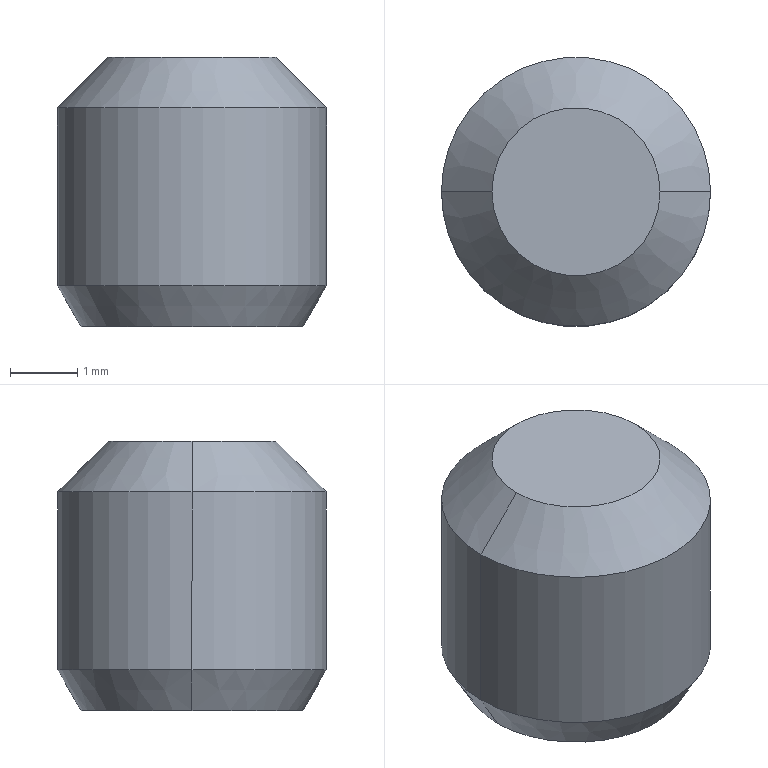Part | SolidWorks | features BaseBody 1 | 1 solid | 15 faces | box 4 x 4 x 4 mm | volume 40.721 mm3 | plane 9 | cone 4 | cylinder 2 | commonest cylinder face diameters 4 x2
STEP:
#1=CARTESIAN_POINT('',(461.064,-93.168,231.151));
#2=VERTEX_POINT('',#1);
#3=CARTESIAN_POINT('',(457.064,-93.168,231.151));
#4=VERTEX_POINT('',#3);
#5=CARTESIAN_POINT('',(459.064,-93.168,231.151));
#6=DIRECTION('',(0.000000024,-0.000000004,1.));
#7=DIRECTION('',(1.,0.,-0.000000024));
#8=AXIS2_PLACEMENT_3D('',#5,#6,#7);
#9=CIRCLE('',#8,2.);
#10=EDGE_CURVE('',#2,#4,#9,.T.);
#11=ORIENTED_EDGE('',*,*,#10,.T.);
#12=CARTESIAN_POINT('',(457.064,-93.168,233.795));
#13=VERTEX_POINT('',#12);
#14=CARTESIAN_POINT('',(457.064,-93.168,232.473));
#15=DIRECTION('',(0.000000024,-0.000000004,1.));
#16=VECTOR('',#15,1000.);
#17=LINE('',#14,#16);
#18=EDGE_CURVE('',#4,#13,#17,.T.);
#19=ORIENTED_EDGE('',*,*,#18,.T.);
#20=CARTESIAN_POINT('',(461.064,-93.168,233.795));
#21=VERTEX_POINT('',#20);
#22=CARTESIAN_POINT('',(459.064,-93.168,233.795));
#23=DIRECTION('',(-0.000000024,0.000000004,-1.));
#24=DIRECTION('',(1.,0.,-0.000000024));
#25=AXIS2_PLACEMENT_3D('',#22,#23,#24);
#26=CIRCLE('',#25,2.);
#27=EDGE_CURVE('',#13,#21,#26,.T.);
#28=ORIENTED_EDGE('',*,*,#27,.T.);
#29=CARTESIAN_POINT('',(461.064,-93.168,232.473));
#30=DIRECTION('',(0.000000024,-0.000000004,1.));
#31=VECTOR('',#30,1000.);
#32=LINE('',#29,#31);
#33=EDGE_CURVE('',#2,#21,#32,.T.);
#34=ORIENTED_EDGE('',*,*,#33,.F.);
#35=EDGE_LOOP('',(#11,#19,#28,#34));
#36=FACE_OUTER_BOUND('',#35,.T.);
#37=CARTESIAN_POINT('',(459.064,-93.168,232.473));
#38=DIRECTION('',(0.000000024,-0.000000004,1.));
#39=DIRECTION('',(1.,0.,-0.000000024));
#40=AXIS2_PLACEMENT_3D('',#37,#38,#39);
#41=CYLINDRICAL_SURFACE('',#40,2.);
#42=ADVANCED_FACE('',(#36),#41,.T.);
#43=CARTESIAN_POINT('',(460.714,-93.168,230.545));
#44=VERTEX_POINT('',#43);
#45=CARTESIAN_POINT('',(457.414,-93.168,230.545));
#46=VERTEX_POINT('',#45);
#47=CARTESIAN_POINT('',(459.064,-93.168,230.545));
#48=DIRECTION('',(0.000000024,-0.000000004,1.));
#49=DIRECTION('',(1.,0.,-0.000000024));
#50=AXIS2_PLACEMENT_3D('',#47,#48,#49);
#51=CIRCLE('',#50,1.65);
#52=EDGE_CURVE('',#44,#46,#51,.T.);
#53=ORIENTED_EDGE('',*,*,#52,.T.);
#54=CARTESIAN_POINT('',(457.064,-93.168,231.151));
#55=DIRECTION('',(-0.5,-0.000000003,0.866));
#56=VECTOR('',#55,1000.);
#57=LINE('',#54,#56);
#58=EDGE_CURVE('',#46,#4,#57,.T.);
#59=ORIENTED_EDGE('',*,*,#58,.T.);
#60=ORIENTED_EDGE('',*,*,#10,.F.);
#61=CARTESIAN_POINT('',(461.064,-93.168,231.151));
#62=DIRECTION('',(0.5,-0.000000003,0.866));
#63=VECTOR('',#62,1000.);
#64=LINE('',#61,#63);
#65=EDGE_CURVE('',#44,#2,#64,.T.);
#66=ORIENTED_EDGE('',*,*,#65,.F.);
#67=EDGE_LOOP('',(#53,#59,#60,#66));
#68=FACE_OUTER_BOUND('',#67,.T.);
#69=CARTESIAN_POINT('',(459.064,-93.168,231.151));
#70=DIRECTION('',(0.000000024,-0.000000004,1.));
#71=DIRECTION('',(1.,0.,-0.000000024));
#72=AXIS2_PLACEMENT_3D('',#69,#70,#71);
#73=CONICAL_SURFACE('',#72,2.,0.5236);
#74=ADVANCED_FACE('',(#68),#73,.T.);
#75=CARTESIAN_POINT('',(457.814,-93.168,234.545));
#76=VERTEX_POINT('',#75);
#77=CARTESIAN_POINT('',(460.314,-93.168,234.545));
#78=VERTEX_POINT('',#77);
#79=CARTESIAN_POINT('',(459.064,-93.168,234.545));
#80=DIRECTION('',(-0.000000024,0.000000004,-1.));
#81=DIRECTION('',(-1.,0.,0.000000024));
#82=AXIS2_PLACEMENT_3D('',#79,#80,#81);
#83=CIRCLE('',#82,1.25);
#84=EDGE_CURVE('',#76,#78,#83,.T.);
#85=ORIENTED_EDGE('',*,*,#84,.T.);
#86=CARTESIAN_POINT('',(461.064,-93.168,233.795));
#87=DIRECTION('',(0.7071,0.000000003,-0.7071));
#88=VECTOR('',#87,1000.);
#89=LINE('',#86,#88);
#90=EDGE_CURVE('',#78,#21,#89,.T.);
#91=ORIENTED_EDGE('',*,*,#90,.T.);
#92=ORIENTED_EDGE('',*,*,#27,.F.);
#93=CARTESIAN_POINT('',(457.064,-93.168,233.795));
#94=DIRECTION('',(-0.7071,0.000000003,-0.7071));
#95=VECTOR('',#94,1000.);
#96=LINE('',#93,#95);
#97=EDGE_CURVE('',#76,#13,#96,.T.);
#98=ORIENTED_EDGE('',*,*,#97,.F.);
#99=EDGE_LOOP('',(#85,#91,#92,#98));
#100=FACE_OUTER_BOUND('',#99,.T.);
#101=CARTESIAN_POINT('',(459.064,-93.168,233.795));
#102=DIRECTION('',(-0.000000024,0.000000004,-1.));
#103=DIRECTION('',(-1.,0.,0.000000024));
#104=AXIS2_PLACEMENT_3D('',#101,#102,#103);
#105=CONICAL_SURFACE('',#104,2.,0.7854);
#106=ADVANCED_FACE('',(#100),#105,.T.);
#107=ORIENTED_EDGE('',*,*,#18,.F.);
#108=CARTESIAN_POINT('',(459.064,-93.168,231.151));
#109=DIRECTION('',(0.000000024,-0.000000004,1.));
#110=DIRECTION('',(1.,0.,-0.000000024));
#111=AXIS2_PLACEMENT_3D('',#108,#109,#110);
#112=CIRCLE('',#111,2.);
#113=EDGE_CURVE('',#4,#2,#112,.T.);
#114=ORIENTED_EDGE('',*,*,#113,.T.);
#115=ORIENTED_EDGE('',*,*,#33,.T.);
#116=CARTESIAN_POINT('',(459.064,-93.168,233.795));
#117=DIRECTION('',(-0.000000024,0.000000004,-1.));
#118=DIRECTION('',(1.,0.,-0.000000024));
#119=AXIS2_PLACEMENT_3D('',#116,#117,#118);
#120=CIRCLE('',#119,2.);
#121=EDGE_CURVE('',#21,#13,#120,.T.);
#122=ORIENTED_EDGE('',*,*,#121,.T.);
#123=EDGE_LOOP('',(#107,#114,#115,#122));
#124=FACE_OUTER_BOUND('',#123,.T.);
#125=CARTESIAN_POINT('',(459.064,-93.168,232.473));
#126=DIRECTION('',(0.000000024,-0.000000004,1.));
#127=DIRECTION('',(1.,0.,-0.000000024));
#128=AXIS2_PLACEMENT_3D('',#125,#126,#127);
#129=CYLINDRICAL_SURFACE('',#128,2.);
#130=ADVANCED_FACE('',(#124),#129,.T.);
#131=ORIENTED_EDGE('',*,*,#58,.F.);
#132=CARTESIAN_POINT('',(459.064,-93.168,230.545));
#133=DIRECTION('',(0.000000024,-0.000000004,1.));
#134=DIRECTION('',(1.,0.,-0.000000024));
#135=AXIS2_PLACEMENT_3D('',#132,#133,#134);
#136=CIRCLE('',#135,1.65);
#137=EDGE_CURVE('',#46,#44,#136,.T.);
#138=ORIENTED_EDGE('',*,*,#137,.T.);
#139=ORIENTED_EDGE('',*,*,#65,.T.);
#140=ORIENTED_EDGE('',*,*,#113,.F.);
#141=EDGE_LOOP('',(#131,#138,#139,#140));
#142=FACE_OUTER_BOUND('',#141,.T.);
#143=CARTESIAN_POINT('',(459.064,-93.168,231.151));
#144=DIRECTION('',(0.000000024,-0.000000004,1.));
#145=DIRECTION('',(1.,0.,-0.000000024));
#146=AXIS2_PLACEMENT_3D('',#143,#144,#145);
#147=CONICAL_SURFACE('',#146,2.,0.5236);
#148=ADVANCED_FACE('',(#142),#147,.T.);
#149=ORIENTED_EDGE('',*,*,#90,.F.);
#150=CARTESIAN_POINT('',(459.064,-93.168,234.545));
#151=DIRECTION('',(-0.000000024,0.000000004,-1.));
#152=DIRECTION('',(-1.,0.,0.000000024));
#153=AXIS2_PLACEMENT_3D('',#150,#151,#152);
#154=CIRCLE('',#153,1.25);
#155=EDGE_CURVE('',#78,#76,#154,.T.);
#156=ORIENTED_EDGE('',*,*,#155,.T.);
#157=ORIENTED_EDGE('',*,*,#97,.T.);
#158=ORIENTED_EDGE('',*,*,#121,.F.);
#159=EDGE_LOOP('',(#149,#156,#157,#158));
#160=FACE_OUTER_BOUND('',#159,.T.);
#161=CARTESIAN_POINT('',(459.064,-93.168,233.795));
#162=DIRECTION('',(-0.000000024,0.000000004,-1.));
#163=DIRECTION('',(-1.,0.,0.000000024));
#164=AXIS2_PLACEMENT_3D('',#161,#162,#163);
#165=CONICAL_SURFACE('',#164,2.,0.7854);
#166=ADVANCED_FACE('',(#160),#165,.T.);
#167=ORIENTED_EDGE('',*,*,#52,.F.);
#168=ORIENTED_EDGE('',*,*,#137,.F.);
#169=EDGE_LOOP('',(#167,#168));
#170=FACE_OUTER_BOUND('',#169,.T.);
#171=CARTESIAN_POINT('',(458.881,-94.308,230.545));
#172=VERTEX_POINT('',#171);
#173=CARTESIAN_POINT('',(459.959,-93.896,230.545));
#174=VERTEX_POINT('',#173);
#175=CARTESIAN_POINT('',(458.881,-94.308,230.545));
#176=DIRECTION('',(0.9343,0.3564,-0.000000021));
#177=VECTOR('',#176,1000.);
#178=LINE('',#175,#177);
#179=EDGE_CURVE('',#172,#174,#178,.T.);
#180=ORIENTED_EDGE('',*,*,#179,.T.);
#181=CARTESIAN_POINT('',(460.142,-92.756,230.545));
#182=VERTEX_POINT('',#181);
#183=CARTESIAN_POINT('',(459.959,-93.896,230.545));
#184=DIRECTION('',(0.1585,0.9874,0.));
#185=VECTOR('',#184,1000.);
#186=LINE('',#183,#185);
#187=EDGE_CURVE('',#174,#182,#186,.T.);
#188=ORIENTED_EDGE('',*,*,#187,.T.);
#189=CARTESIAN_POINT('',(459.247,-92.027,230.545));
#190=VERTEX_POINT('',#189);
#191=CARTESIAN_POINT('',(460.142,-92.756,230.545));
#192=DIRECTION('',(-0.7758,0.6309,0.000000021));
#193=VECTOR('',#192,1000.);
#194=LINE('',#191,#193);
#195=EDGE_CURVE('',#182,#190,#194,.T.);
#196=ORIENTED_EDGE('',*,*,#195,.T.);
#197=CARTESIAN_POINT('',(458.168,-92.439,230.545));
#198=VERTEX_POINT('',#197);
#199=CARTESIAN_POINT('',(459.247,-92.027,230.545));
#200=DIRECTION('',(-0.9343,-0.3564,0.000000021));
#201=VECTOR('',#200,1000.);
#202=LINE('',#199,#201);
#203=EDGE_CURVE('',#190,#198,#202,.T.);
#204=ORIENTED_EDGE('',*,*,#203,.T.);
#205=CARTESIAN_POINT('',(457.985,-93.579,230.545));
#206=VERTEX_POINT('',#205);
#207=CARTESIAN_POINT('',(458.168,-92.439,230.545));
#208=DIRECTION('',(-0.1585,-0.9874,0.));
#209=VECTOR('',#208,1000.);
#210=LINE('',#207,#209);
#211=EDGE_CURVE('',#198,#206,#210,.T.);
#212=ORIENTED_EDGE('',*,*,#211,.T.);
#213=CARTESIAN_POINT('',(457.985,-93.579,230.545));
#214=DIRECTION('',(0.7758,-0.6309,-0.000000021));
#215=VECTOR('',#214,1000.);
#216=LINE('',#213,#215);
#217=EDGE_CURVE('',#206,#172,#216,.T.);
#218=ORIENTED_EDGE('',*,*,#217,.T.);
#219=EDGE_LOOP('',(#180,#188,#196,#204,#212,#218));
#220=FACE_BOUND('',#219,.T.);
#221=CARTESIAN_POINT('',(458.423,-92.647,230.545));
#222=DIRECTION('',(-0.000000024,0.000000004,-1.));
#223=DIRECTION('',(-1.,0.,0.000000024));
#224=AXIS2_PLACEMENT_3D('',#221,#222,#223);
#225=PLANE('',#224);
#226=ADVANCED_FACE('',(#170,#220),#225,.T.);
#227=ORIENTED_EDGE('',*,*,#84,.F.);
#228=ORIENTED_EDGE('',*,*,#155,.F.);
#229=EDGE_LOOP('',(#227,#228));
#230=FACE_OUTER_BOUND('',#229,.T.);
#231=CARTESIAN_POINT('',(458.579,-92.773,234.545));
#232=DIRECTION('',(0.000000024,-0.000000004,1.));
#233=DIRECTION('',(1.,0.,-0.000000024));
#234=AXIS2_PLACEMENT_3D('',#231,#232,#233);
#235=PLANE('',#234);
#236=ADVANCED_FACE('',(#230),#235,.T.);
#237=CARTESIAN_POINT('',(460.142,-92.756,232.045));
#238=VERTEX_POINT('',#237);
#239=CARTESIAN_POINT('',(460.142,-92.756,230.545));
#240=DIRECTION('',(0.000000024,-0.000000004,1.));
#241=VECTOR('',#240,1000.);
#242=LINE('',#239,#241);
#243=EDGE_CURVE('',#182,#238,#242,.T.);
#244=ORIENTED_EDGE('',*,*,#243,.F.);
#245=ORIENTED_EDGE('',*,*,#187,.F.);
#246=CARTESIAN_POINT('',(459.959,-93.896,232.045));
#247=VERTEX_POINT('',#246);
#248=CARTESIAN_POINT('',(459.959,-93.896,230.545));
#249=DIRECTION('',(-0.000000024,0.000000004,-1.));
#250=VECTOR('',#249,1000.);
#251=LINE('',#248,#250);
#252=EDGE_CURVE('',#247,#174,#251,.T.);
#253=ORIENTED_EDGE('',*,*,#252,.F.);
#254=CARTESIAN_POINT('',(460.142,-92.756,232.045));
#255=DIRECTION('',(-0.1585,-0.9874,0.));
#256=VECTOR('',#255,1000.);
#257=LINE('',#254,#256);
#258=EDGE_CURVE('',#238,#247,#257,.T.);
#259=ORIENTED_EDGE('',*,*,#258,.F.);
#260=EDGE_LOOP('',(#244,#245,#253,#259));
#261=FACE_OUTER_BOUND('',#260,.T.);
#262=CARTESIAN_POINT('',(460.142,-92.756,230.545));
#263=DIRECTION('',(0.9874,-0.1585,-0.000000024));
#264=DIRECTION('',(0.1585,0.9874,0.));
#265=AXIS2_PLACEMENT_3D('',#262,#263,#264);
#266=PLANE('',#265);
#267=ADVANCED_FACE('',(#261),#266,.F.);
#268=ORIENTED_EDGE('',*,*,#252,.T.);
#269=ORIENTED_EDGE('',*,*,#179,.F.);
#270=CARTESIAN_POINT('',(458.881,-94.308,232.045));
#271=VERTEX_POINT('',#270);
#272=CARTESIAN_POINT('',(458.881,-94.308,230.545));
#273=DIRECTION('',(-0.000000004,0.000000011,-1.));
#274=VECTOR('',#273,1000.);
#275=LINE('',#272,#274);
#276=EDGE_CURVE('',#271,#172,#275,.T.);
#277=ORIENTED_EDGE('',*,*,#276,.F.);
#278=CARTESIAN_POINT('',(459.959,-93.896,232.045));
#279=DIRECTION('',(-0.9343,-0.3564,0.));
#280=VECTOR('',#279,1000.);
#281=LINE('',#278,#280);
#282=EDGE_CURVE('',#247,#271,#281,.T.);
#283=ORIENTED_EDGE('',*,*,#282,.F.);
#284=EDGE_LOOP('',(#268,#269,#277,#283));
#285=FACE_OUTER_BOUND('',#284,.T.);
#286=CARTESIAN_POINT('',(459.959,-93.896,230.545));
#287=DIRECTION('',(0.3564,-0.9343,-0.000000012));
#288=DIRECTION('',(0.9343,0.3564,0.));
#289=AXIS2_PLACEMENT_3D('',#286,#287,#288);
#290=PLANE('',#289);
#291=ADVANCED_FACE('',(#285),#290,.F.);
#292=ORIENTED_EDGE('',*,*,#276,.T.);
#293=ORIENTED_EDGE('',*,*,#217,.F.);
#294=CARTESIAN_POINT('',(457.985,-93.579,232.045));
#295=VERTEX_POINT('',#294);
#296=CARTESIAN_POINT('',(457.985,-93.579,230.545));
#297=DIRECTION('',(-0.000000008,-0.000000009,-1.));
#298=VECTOR('',#297,1000.);
#299=LINE('',#296,#298);
#300=EDGE_CURVE('',#295,#206,#299,.T.);
#301=ORIENTED_EDGE('',*,*,#300,.F.);
#302=CARTESIAN_POINT('',(458.881,-94.308,232.045));
#303=DIRECTION('',(-0.7758,0.6309,0.));
#304=VECTOR('',#303,1000.);
#305=LINE('',#302,#304);
#306=EDGE_CURVE('',#271,#295,#305,.T.);
#307=ORIENTED_EDGE('',*,*,#306,.F.);
#308=EDGE_LOOP('',(#292,#293,#301,#307));
#309=FACE_OUTER_BOUND('',#308,.T.);
#310=CARTESIAN_POINT('',(458.881,-94.308,230.545));
#311=DIRECTION('',(-0.6309,-0.7758,0.000000012));
#312=DIRECTION('',(0.7758,-0.6309,0.));
#313=AXIS2_PLACEMENT_3D('',#310,#311,#312);
#314=PLANE('',#313);
#315=ADVANCED_FACE('',(#309),#314,.F.);
#316=ORIENTED_EDGE('',*,*,#300,.T.);
#317=ORIENTED_EDGE('',*,*,#211,.F.);
#318=CARTESIAN_POINT('',(458.168,-92.439,232.045));
#319=VERTEX_POINT('',#318);
#320=CARTESIAN_POINT('',(458.168,-92.439,230.545));
#321=DIRECTION('',(-0.000000024,0.000000004,-1.));
#322=VECTOR('',#321,1000.);
#323=LINE('',#320,#322);
#324=EDGE_CURVE('',#319,#198,#323,.T.);
#325=ORIENTED_EDGE('',*,*,#324,.F.);
#326=CARTESIAN_POINT('',(457.985,-93.579,232.045));
#327=DIRECTION('',(0.1585,0.9874,0.));
#328=VECTOR('',#327,1000.);
#329=LINE('',#326,#328);
#330=EDGE_CURVE('',#295,#319,#329,.T.);
#331=ORIENTED_EDGE('',*,*,#330,.F.);
#332=EDGE_LOOP('',(#316,#317,#325,#331));
#333=FACE_OUTER_BOUND('',#332,.T.);
#334=CARTESIAN_POINT('',(457.985,-93.579,230.545));
#335=DIRECTION('',(-0.9874,0.1585,0.000000024));
#336=DIRECTION('',(-0.1585,-0.9874,0.));
#337=AXIS2_PLACEMENT_3D('',#334,#335,#336);
#338=PLANE('',#337);
#339=ADVANCED_FACE('',(#333),#338,.F.);
#340=ORIENTED_EDGE('',*,*,#324,.T.);
#341=ORIENTED_EDGE('',*,*,#203,.F.);
#342=CARTESIAN_POINT('',(459.247,-92.027,232.045));
#343=VERTEX_POINT('',#342);
#344=CARTESIAN_POINT('',(459.247,-92.027,230.545));
#345=DIRECTION('',(-0.000000004,0.000000011,-1.));
#346=VECTOR('',#345,1000.);
#347=LINE('',#344,#346);
#348=EDGE_CURVE('',#343,#190,#347,.T.);
#349=ORIENTED_EDGE('',*,*,#348,.F.);
#350=CARTESIAN_POINT('',(458.168,-92.439,232.045));
#351=DIRECTION('',(0.9343,0.3564,0.));
#352=VECTOR('',#351,1000.);
#353=LINE('',#350,#352);
#354=EDGE_CURVE('',#319,#343,#353,.T.);
#355=ORIENTED_EDGE('',*,*,#354,.F.);
#356=EDGE_LOOP('',(#340,#341,#349,#355));
#357=FACE_OUTER_BOUND('',#356,.T.);
#358=CARTESIAN_POINT('',(458.168,-92.439,230.545));
#359=DIRECTION('',(-0.3564,0.9343,0.000000012));
#360=DIRECTION('',(-0.9343,-0.3564,0.));
#361=AXIS2_PLACEMENT_3D('',#358,#359,#360);
#362=PLANE('',#361);
#363=ADVANCED_FACE('',(#357),#362,.F.);
#364=ORIENTED_EDGE('',*,*,#348,.T.);
#365=ORIENTED_EDGE('',*,*,#195,.F.);
#366=ORIENTED_EDGE('',*,*,#243,.T.);
#367=CARTESIAN_POINT('',(459.247,-92.027,232.045));
#368=DIRECTION('',(0.7758,-0.6309,0.));
#369=VECTOR('',#368,1000.);
#370=LINE('',#367,#369);
#371=EDGE_CURVE('',#343,#238,#370,.T.);
#372=ORIENTED_EDGE('',*,*,#371,.F.);
#373=EDGE_LOOP('',(#364,#365,#366,#372));
#374=FACE_OUTER_BOUND('',#373,.T.);
#375=CARTESIAN_POINT('',(459.247,-92.027,230.545));
#376=DIRECTION('',(0.6309,0.7758,-0.000000012));
#377=DIRECTION('',(-0.7758,0.6309,0.));
#378=AXIS2_PLACEMENT_3D('',#375,#376,#377);
#379=PLANE('',#378);
#380=ADVANCED_FACE('',(#374),#379,.F.);
#381=ORIENTED_EDGE('',*,*,#330,.T.);
#382=ORIENTED_EDGE('',*,*,#354,.T.);
#383=ORIENTED_EDGE('',*,*,#371,.T.);
#384=ORIENTED_EDGE('',*,*,#258,.T.);
#385=ORIENTED_EDGE('',*,*,#282,.T.);
#386=ORIENTED_EDGE('',*,*,#306,.T.);
#387=EDGE_LOOP('',(#381,#382,#383,#384,#385,#386));
#388=FACE_OUTER_BOUND('',#387,.T.);
#389=CARTESIAN_POINT('',(459.064,-93.168,232.045));
#390=DIRECTION('',(-0.000000024,0.000000004,-1.));
#391=DIRECTION('',(-1.,0.,0.000000024));
#392=AXIS2_PLACEMENT_3D('',#389,#390,#391);
#393=PLANE('',#392);
#394=ADVANCED_FACE('',(#388),#393,.T.);
#395=CLOSED_SHELL('',(#42,#74,#106,#130,#148,#166,#226,#236,#267,#291,#315,#339,#363,#380,#394));
#396=MANIFOLD_SOLID_BREP('',#395);
#397=CARTESIAN_POINT('',(0.,0.,0.));
#398=DIRECTION('',(0.,0.,1.));
#399=DIRECTION('',(1.,0.,0.));
#400=AXIS2_PLACEMENT_3D('',#397,#398,#399);
#401=(LENGTH_UNIT()NAMED_UNIT(*)SI_UNIT(.MILLI.,.METRE.));
#402=UNCERTAINTY_MEASURE_WITH_UNIT(LENGTH_MEASURE(0.00001),#401,'','');
#403=(NAMED_UNIT(*)PLANE_ANGLE_UNIT()SI_UNIT($,.RADIAN.));
#404=(NAMED_UNIT(*)SI_UNIT($,.STERADIAN.)SOLID_ANGLE_UNIT());
#405=(GEOMETRIC_REPRESENTATION_CONTEXT(3)GLOBAL_UNCERTAINTY_ASSIGNED_CONTEXT((#402))GLOBAL_UNIT_ASSIGNED_CONTEXT((#401,#403,#404))REPRESENTATION_CONTEXT('',''));
#406=ADVANCED_BREP_SHAPE_REPRESENTATION('',(#396,#400),#405);